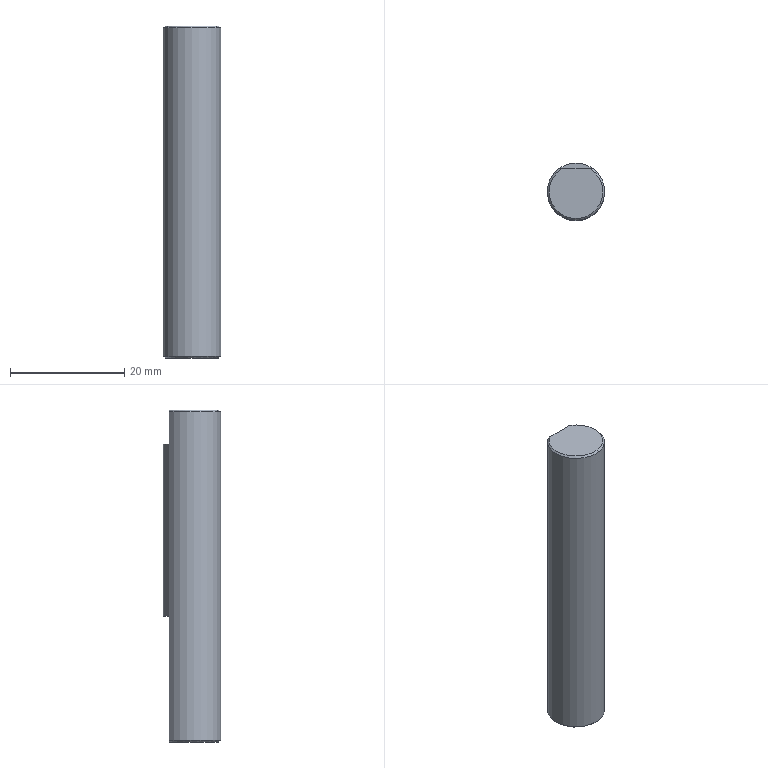Part | NX | features MOVE_FACE 2, BREP 1 | 1 solid | 9 faces | box 10 x 10 x 58 mm | volume 4439 mm3 | plane 6 | cone 2 | cylinder 1 | commonest cylinder face diameters 10 x1
STEP:
#1=CARTESIAN_POINT('',(-3.,4.,-2.3));
#2=VERTEX_POINT('',#1);
#3=CARTESIAN_POINT('',(-2.468,4.,-2.));
#4=VERTEX_POINT('',#3);
#5=CARTESIAN_POINT('',(-3.,4.,-2.3));
#6=CARTESIAN_POINT('',(-2.825,4.,-2.195));
#7=CARTESIAN_POINT('',(-2.648,4.,-2.095));
#8=CARTESIAN_POINT('',(-2.468,4.,-2.));
#9=B_SPLINE_CURVE_WITH_KNOTS('',3,(#5,#6,#7,#8),.UNSPECIFIED.,.F.,.F.,(4,4),(0.009427,0.01004),.UNSPECIFIED.);
#10=EDGE_CURVE('',#2,#4,#9,.T.);
#11=ORIENTED_EDGE('',*,*,#10,.F.);
#12=CARTESIAN_POINT('',(3.,4.,-2.3));
#13=VERTEX_POINT('',#12);
#14=CARTESIAN_POINT('',(0.,0.,-2.3));
#15=DIRECTION('',(0.,0.,-1.));
#16=DIRECTION('',(-1.,0.,0.));
#17=AXIS2_PLACEMENT_3D('',#14,#15,#16);
#18=CIRCLE('',#17,5.);
#19=EDGE_CURVE('',#13,#2,#18,.T.);
#20=ORIENTED_EDGE('',*,*,#19,.F.);
#21=CARTESIAN_POINT('',(2.468,4.,-2.));
#22=VERTEX_POINT('',#21);
#23=CARTESIAN_POINT('',(2.468,4.,-2.));
#24=CARTESIAN_POINT('',(2.648,4.,-2.095));
#25=CARTESIAN_POINT('',(2.825,4.,-2.195));
#26=CARTESIAN_POINT('',(3.,4.,-2.3));
#27=B_SPLINE_CURVE_WITH_KNOTS('',3,(#23,#24,#25,#26),.UNSPECIFIED.,.F.,.F.,(4,4),(0.01523,0.01584),.UNSPECIFIED.);
#28=EDGE_CURVE('',#22,#13,#27,.T.);
#29=ORIENTED_EDGE('',*,*,#28,.F.);
#30=CARTESIAN_POINT('',(0.,0.,-2.));
#31=DIRECTION('',(0.,0.,-1.));
#32=DIRECTION('',(-1.,0.,0.));
#33=AXIS2_PLACEMENT_3D('',#30,#31,#32);
#34=CIRCLE('',#33,4.7);
#35=EDGE_CURVE('',#22,#4,#34,.T.);
#36=ORIENTED_EDGE('',*,*,#35,.T.);
#37=EDGE_LOOP('',(#11,#20,#29,#36));
#38=FACE_BOUND('',#37,.T.);
#39=CARTESIAN_POINT('',(0.,0.,-2.));
#40=DIRECTION('',(0.,0.,-1.));
#41=DIRECTION('',(-1.,0.,0.));
#42=AXIS2_PLACEMENT_3D('',#39,#40,#41);
#43=CONICAL_SURFACE('',#42,4.7,0.7854);
#44=ADVANCED_FACE('',(#38),#43,.T.);
#45=CARTESIAN_POINT('',(3.,4.,-8.));
#46=VERTEX_POINT('',#45);
#47=CARTESIAN_POINT('',(-3.,4.,-8.));
#48=VERTEX_POINT('',#47);
#49=CARTESIAN_POINT('',(0.,0.,-8.));
#50=DIRECTION('',(0.,0.,1.));
#51=DIRECTION('',(1.,0.,0.));
#52=AXIS2_PLACEMENT_3D('',#49,#50,#51);
#53=CIRCLE('',#52,5.);
#54=EDGE_CURVE('',#46,#48,#53,.T.);
#55=ORIENTED_EDGE('',*,*,#54,.F.);
#56=CARTESIAN_POINT('',(3.,4.,-50.));
#57=DIRECTION('',(0.,0.,-1.));
#58=VECTOR('',#57,1000.);
#59=LINE('',#56,#58);
#60=EDGE_CURVE('',#13,#46,#59,.T.);
#61=ORIENTED_EDGE('',*,*,#60,.F.);
#62=ORIENTED_EDGE('',*,*,#19,.T.);
#63=CARTESIAN_POINT('',(-3.,4.,-50.));
#64=DIRECTION('',(0.,0.,-1.));
#65=VECTOR('',#64,1000.);
#66=LINE('',#63,#65);
#67=EDGE_CURVE('',#2,#48,#66,.T.);
#68=ORIENTED_EDGE('',*,*,#67,.T.);
#69=EDGE_LOOP('',(#55,#61,#62,#68));
#70=FACE_BOUND('',#69,.T.);
#71=CARTESIAN_POINT('',(3.,4.,-38.));
#72=VERTEX_POINT('',#71);
#73=CARTESIAN_POINT('',(3.,4.,-59.7));
#74=VERTEX_POINT('',#73);
#75=CARTESIAN_POINT('',(3.,4.,-50.));
#76=DIRECTION('',(0.,0.,-1.));
#77=VECTOR('',#76,1000.);
#78=LINE('',#75,#77);
#79=EDGE_CURVE('',#72,#74,#78,.T.);
#80=ORIENTED_EDGE('',*,*,#79,.F.);
#81=CARTESIAN_POINT('',(-3.,4.,-38.));
#82=VERTEX_POINT('',#81);
#83=CARTESIAN_POINT('',(0.,0.,-38.));
#84=DIRECTION('',(0.,0.,-1.));
#85=DIRECTION('',(-1.,0.,0.));
#86=AXIS2_PLACEMENT_3D('',#83,#84,#85);
#87=CIRCLE('',#86,5.);
#88=EDGE_CURVE('',#82,#72,#87,.T.);
#89=ORIENTED_EDGE('',*,*,#88,.F.);
#90=CARTESIAN_POINT('',(-3.,4.,-59.7));
#91=VERTEX_POINT('',#90);
#92=CARTESIAN_POINT('',(-3.,4.,-50.));
#93=DIRECTION('',(0.,0.,-1.));
#94=VECTOR('',#93,1000.);
#95=LINE('',#92,#94);
#96=EDGE_CURVE('',#82,#91,#95,.T.);
#97=ORIENTED_EDGE('',*,*,#96,.T.);
#98=CARTESIAN_POINT('',(0.,0.,-59.7));
#99=DIRECTION('',(0.,0.,-1.));
#100=DIRECTION('',(-1.,0.,0.));
#101=AXIS2_PLACEMENT_3D('',#98,#99,#100);
#102=CIRCLE('',#101,5.);
#103=EDGE_CURVE('',#74,#91,#102,.T.);
#104=ORIENTED_EDGE('',*,*,#103,.F.);
#105=EDGE_LOOP('',(#80,#89,#97,#104));
#106=FACE_BOUND('',#105,.T.);
#107=CARTESIAN_POINT('',(0.,0.,-50.));
#108=DIRECTION('',(0.,0.,1.));
#109=DIRECTION('',(-1.,0.,0.));
#110=AXIS2_PLACEMENT_3D('',#107,#108,#109);
#111=CYLINDRICAL_SURFACE('',#110,5.);
#112=ADVANCED_FACE('',(#70,#106),#111,.T.);
#113=CARTESIAN_POINT('',(2.468,4.,-60.));
#114=VERTEX_POINT('',#113);
#115=CARTESIAN_POINT('',(3.,4.,-59.7));
#116=CARTESIAN_POINT('',(2.825,4.,-59.805));
#117=CARTESIAN_POINT('',(2.648,4.,-59.905));
#118=CARTESIAN_POINT('',(2.468,4.,-60.));
#119=B_SPLINE_CURVE_WITH_KNOTS('',3,(#115,#116,#117,#118),.UNSPECIFIED.,.F.,.F.,(4,4),(0.009427,0.01004),.UNSPECIFIED.);
#120=EDGE_CURVE('',#74,#114,#119,.T.);
#121=ORIENTED_EDGE('',*,*,#120,.F.);
#122=ORIENTED_EDGE('',*,*,#103,.T.);
#123=CARTESIAN_POINT('',(-2.468,4.,-60.));
#124=VERTEX_POINT('',#123);
#125=CARTESIAN_POINT('',(-2.468,4.,-60.));
#126=CARTESIAN_POINT('',(-2.648,4.,-59.905));
#127=CARTESIAN_POINT('',(-2.825,4.,-59.805));
#128=CARTESIAN_POINT('',(-3.,4.,-59.7));
#129=B_SPLINE_CURVE_WITH_KNOTS('',3,(#125,#126,#127,#128),.UNSPECIFIED.,.F.,.F.,(4,4),(0.01523,0.01584),.UNSPECIFIED.);
#130=EDGE_CURVE('',#124,#91,#129,.T.);
#131=ORIENTED_EDGE('',*,*,#130,.F.);
#132=CARTESIAN_POINT('',(0.,0.,-60.));
#133=DIRECTION('',(0.,0.,-1.));
#134=DIRECTION('',(-1.,0.,0.));
#135=AXIS2_PLACEMENT_3D('',#132,#133,#134);
#136=CIRCLE('',#135,4.7);
#137=EDGE_CURVE('',#114,#124,#136,.T.);
#138=ORIENTED_EDGE('',*,*,#137,.F.);
#139=EDGE_LOOP('',(#121,#122,#131,#138));
#140=FACE_BOUND('',#139,.T.);
#141=CARTESIAN_POINT('',(0.,0.,-59.7));
#142=DIRECTION('',(0.,0.,1.));
#143=DIRECTION('',(1.,0.,0.));
#144=AXIS2_PLACEMENT_3D('',#141,#142,#143);
#145=CONICAL_SURFACE('',#144,5.,0.7854);
#146=ADVANCED_FACE('',(#140),#145,.T.);
#147=ORIENTED_EDGE('',*,*,#35,.F.);
#148=CARTESIAN_POINT('',(10.,4.,-2.));
#149=DIRECTION('',(-1.,0.,0.));
#150=VECTOR('',#149,1000.);
#151=LINE('',#148,#150);
#152=EDGE_CURVE('',#22,#4,#151,.T.);
#153=ORIENTED_EDGE('',*,*,#152,.T.);
#154=EDGE_LOOP('',(#147,#153));
#155=FACE_BOUND('',#154,.T.);
#156=CARTESIAN_POINT('',(0.,0.,-2.));
#157=DIRECTION('',(0.,0.,-1.));
#158=DIRECTION('',(-1.,0.,0.));
#159=AXIS2_PLACEMENT_3D('',#156,#157,#158);
#160=PLANE('',#159);
#161=ADVANCED_FACE('',(#155),#160,.F.);
#162=CARTESIAN_POINT('',(0.,4.,-60.));
#163=DIRECTION('',(-1.,0.,0.));
#164=VECTOR('',#163,1000.);
#165=LINE('',#162,#164);
#166=EDGE_CURVE('',#114,#124,#165,.T.);
#167=ORIENTED_EDGE('',*,*,#166,.F.);
#168=ORIENTED_EDGE('',*,*,#137,.T.);
#169=EDGE_LOOP('',(#167,#168));
#170=FACE_BOUND('',#169,.T.);
#171=CARTESIAN_POINT('',(0.,4.7,-60.));
#172=DIRECTION('',(0.,0.,1.));
#173=DIRECTION('',(1.,0.,0.));
#174=AXIS2_PLACEMENT_3D('',#171,#172,#173);
#175=PLANE('',#174);
#176=ADVANCED_FACE('',(#170),#175,.F.);
#177=ORIENTED_EDGE('',*,*,#28,.T.);
#178=ORIENTED_EDGE('',*,*,#60,.T.);
#179=CARTESIAN_POINT('',(10.,4.,-8.));
#180=DIRECTION('',(-1.,0.,0.));
#181=VECTOR('',#180,1000.);
#182=LINE('',#179,#181);
#183=EDGE_CURVE('',#46,#48,#182,.T.);
#184=ORIENTED_EDGE('',*,*,#183,.T.);
#185=ORIENTED_EDGE('',*,*,#67,.F.);
#186=ORIENTED_EDGE('',*,*,#10,.T.);
#187=ORIENTED_EDGE('',*,*,#152,.F.);
#188=EDGE_LOOP('',(#177,#178,#184,#185,#186,#187));
#189=FACE_BOUND('',#188,.T.);
#190=CARTESIAN_POINT('',(10.,4.,0.));
#191=DIRECTION('',(0.,1.,0.));
#192=DIRECTION('',(0.,0.,1.));
#193=AXIS2_PLACEMENT_3D('',#190,#191,#192);
#194=PLANE('',#193);
#195=ADVANCED_FACE('',(#189),#194,.T.);
#196=ORIENTED_EDGE('',*,*,#183,.F.);
#197=ORIENTED_EDGE('',*,*,#54,.T.);
#198=EDGE_LOOP('',(#196,#197));
#199=FACE_BOUND('',#198,.T.);
#200=CARTESIAN_POINT('',(10.,4.,-8.));
#201=DIRECTION('',(0.,0.,1.));
#202=DIRECTION('',(1.,0.,0.));
#203=AXIS2_PLACEMENT_3D('',#200,#201,#202);
#204=PLANE('',#203);
#205=ADVANCED_FACE('',(#199),#204,.T.);
#206=ORIENTED_EDGE('',*,*,#88,.T.);
#207=CARTESIAN_POINT('',(10.,4.,-38.));
#208=DIRECTION('',(-1.,0.,0.));
#209=VECTOR('',#208,1000.);
#210=LINE('',#207,#209);
#211=EDGE_CURVE('',#72,#82,#210,.T.);
#212=ORIENTED_EDGE('',*,*,#211,.T.);
#213=EDGE_LOOP('',(#206,#212));
#214=FACE_BOUND('',#213,.T.);
#215=CARTESIAN_POINT('',(10.,5.,-38.));
#216=DIRECTION('',(0.,0.,-1.));
#217=DIRECTION('',(-1.,0.,0.));
#218=AXIS2_PLACEMENT_3D('',#215,#216,#217);
#219=PLANE('',#218);
#220=ADVANCED_FACE('',(#214),#219,.T.);
#221=ORIENTED_EDGE('',*,*,#79,.T.);
#222=ORIENTED_EDGE('',*,*,#120,.T.);
#223=ORIENTED_EDGE('',*,*,#166,.T.);
#224=ORIENTED_EDGE('',*,*,#130,.T.);
#225=ORIENTED_EDGE('',*,*,#96,.F.);
#226=ORIENTED_EDGE('',*,*,#211,.F.);
#227=EDGE_LOOP('',(#221,#222,#223,#224,#225,#226));
#228=FACE_BOUND('',#227,.T.);
#229=CARTESIAN_POINT('',(10.,4.,-35.));
#230=DIRECTION('',(0.,1.,0.));
#231=DIRECTION('',(0.,0.,1.));
#232=AXIS2_PLACEMENT_3D('',#229,#230,#231);
#233=PLANE('',#232);
#234=ADVANCED_FACE('',(#228),#233,.T.);
#235=CLOSED_SHELL('',(#44,#112,#146,#161,#176,#195,#205,#220,#234));
#236=MANIFOLD_SOLID_BREP('',#235);
#237=(LENGTH_UNIT()NAMED_UNIT(*)SI_UNIT(.MILLI.,.METRE.));
#238=UNCERTAINTY_MEASURE_WITH_UNIT(LENGTH_MEASURE(0.00001),#237,'','');
#239=(NAMED_UNIT(*)PLANE_ANGLE_UNIT()SI_UNIT($,.RADIAN.));
#240=(NAMED_UNIT(*)SI_UNIT($,.STERADIAN.)SOLID_ANGLE_UNIT());
#241=(GEOMETRIC_REPRESENTATION_CONTEXT(3)GLOBAL_UNCERTAINTY_ASSIGNED_CONTEXT((#238))GLOBAL_UNIT_ASSIGNED_CONTEXT((#237,#239,#240))REPRESENTATION_CONTEXT('',''));
#242=ADVANCED_BREP_SHAPE_REPRESENTATION('',(#236),#241);